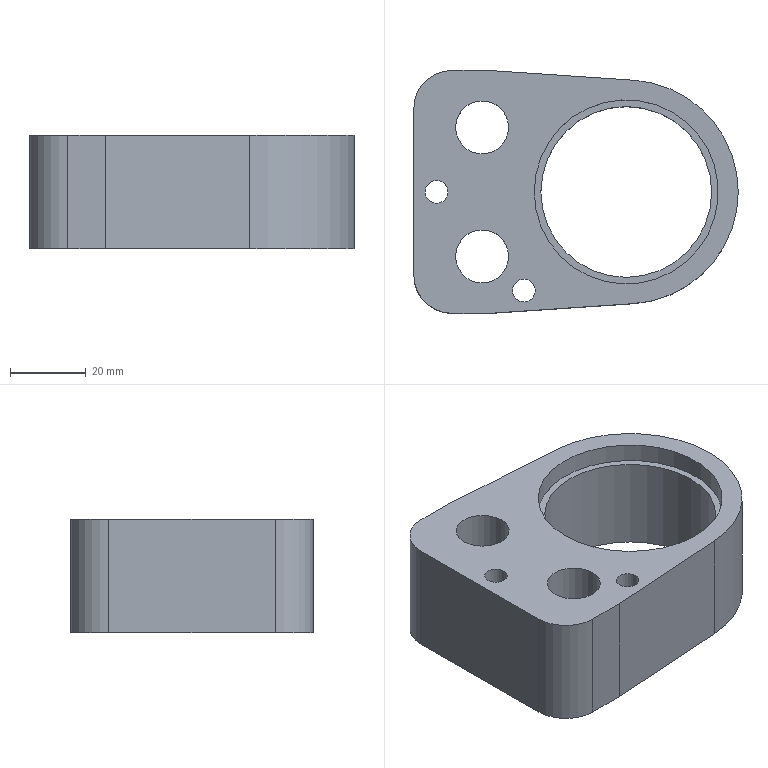Part | NX | features solid 2 | 1 solid | 25 faces | box 85.5 x 64 x 30 mm | volume 80178 mm3 | cylinder 13 | plane 12 | commonest cylinder face diameters 6 x2 8 x2 14 x2 19 x2 20 x2 45 x1
STEP:
#1=CARTESIAN_POINT('',(49.,45.006,17.));
#2=VERTEX_POINT('',#1);
#3=CARTESIAN_POINT('',(45.,45.006,17.));
#4=DIRECTION('',(0.,0.,1.));
#5=DIRECTION('',(1.,0.,0.));
#6=AXIS2_PLACEMENT_3D('',#3,#4,#5);
#7=CIRCLE('',#6,4.);
#8=EDGE_CURVE('',#2,#2,#7,.F.);
#9=ORIENTED_EDGE('',*,*,#8,.F.);
#10=EDGE_LOOP('',(#9));
#11=FACE_BOUND('',#10,.T.);
#12=CARTESIAN_POINT('',(47.5,28.006,17.));
#13=VERTEX_POINT('',#12);
#14=CARTESIAN_POINT('',(57.,28.006,17.));
#15=DIRECTION('',(0.,0.,-1.));
#16=DIRECTION('',(-1.,0.,0.));
#17=AXIS2_PLACEMENT_3D('',#14,#15,#16);
#18=CIRCLE('',#17,9.5);
#19=EDGE_CURVE('',#13,#13,#18,.T.);
#20=ORIENTED_EDGE('',*,*,#19,.F.);
#21=EDGE_LOOP('',(#20));
#22=FACE_BOUND('',#21,.T.);
#23=CARTESIAN_POINT('',(47.5,62.006,17.));
#24=VERTEX_POINT('',#23);
#25=CARTESIAN_POINT('',(57.,62.006,17.));
#26=DIRECTION('',(0.,0.,-1.));
#27=DIRECTION('',(-1.,0.,0.));
#28=AXIS2_PLACEMENT_3D('',#25,#26,#27);
#29=CIRCLE('',#28,9.5);
#30=EDGE_CURVE('',#24,#24,#29,.T.);
#31=ORIENTED_EDGE('',*,*,#30,.F.);
#32=EDGE_LOOP('',(#31));
#33=FACE_BOUND('',#32,.T.);
#34=CARTESIAN_POINT('',(117.5,45.006,17.));
#35=VERTEX_POINT('',#34);
#36=CARTESIAN_POINT('',(95.,45.006,17.));
#37=DIRECTION('',(0.,0.,1.));
#38=DIRECTION('',(1.,0.,0.));
#39=AXIS2_PLACEMENT_3D('',#36,#37,#38);
#40=CIRCLE('',#39,22.5);
#41=EDGE_CURVE('',#35,#35,#40,.T.);
#42=ORIENTED_EDGE('',*,*,#41,.T.);
#43=EDGE_LOOP('',(#42));
#44=FACE_BOUND('',#43,.T.);
#45=CARTESIAN_POINT('',(96.989,74.439,17.));
#46=VERTEX_POINT('',#45);
#47=CARTESIAN_POINT('',(59.,77.006,17.));
#48=VERTEX_POINT('',#47);
#49=CARTESIAN_POINT('',(96.989,74.439,17.));
#50=DIRECTION('',(-0.9977,0.06742,0.));
#51=VECTOR('',#50,1000.);
#52=LINE('',#49,#51);
#53=EDGE_CURVE('',#46,#48,#52,.T.);
#54=ORIENTED_EDGE('',*,*,#53,.F.);
#55=CARTESIAN_POINT('',(96.989,15.574,17.));
#56=VERTEX_POINT('',#55);
#57=CARTESIAN_POINT('',(95.,45.006,17.));
#58=DIRECTION('',(0.,0.,-1.));
#59=DIRECTION('',(-1.,0.,0.));
#60=AXIS2_PLACEMENT_3D('',#57,#58,#59);
#61=CIRCLE('',#60,29.5);
#62=EDGE_CURVE('',#46,#56,#61,.T.);
#63=ORIENTED_EDGE('',*,*,#62,.T.);
#64=CARTESIAN_POINT('',(59.,13.006,17.));
#65=VERTEX_POINT('',#64);
#66=CARTESIAN_POINT('',(96.989,15.574,17.));
#67=DIRECTION('',(-0.9977,-0.06742,0.));
#68=VECTOR('',#67,1000.);
#69=LINE('',#66,#68);
#70=EDGE_CURVE('',#56,#65,#69,.T.);
#71=ORIENTED_EDGE('',*,*,#70,.T.);
#72=CARTESIAN_POINT('',(49.,13.006,17.));
#73=VERTEX_POINT('',#72);
#74=CARTESIAN_POINT('',(59.,13.006,17.));
#75=DIRECTION('',(-1.,0.,0.));
#76=VECTOR('',#75,1000.);
#77=LINE('',#74,#76);
#78=EDGE_CURVE('',#65,#73,#77,.T.);
#79=ORIENTED_EDGE('',*,*,#78,.T.);
#80=CARTESIAN_POINT('',(39.,23.006,17.));
#81=VERTEX_POINT('',#80);
#82=CARTESIAN_POINT('',(49.,23.006,17.));
#83=DIRECTION('',(0.,0.,-1.));
#84=DIRECTION('',(-1.,0.,0.));
#85=AXIS2_PLACEMENT_3D('',#82,#83,#84);
#86=CIRCLE('',#85,10.);
#87=EDGE_CURVE('',#73,#81,#86,.T.);
#88=ORIENTED_EDGE('',*,*,#87,.T.);
#89=CARTESIAN_POINT('',(39.,67.006,17.));
#90=VERTEX_POINT('',#89);
#91=CARTESIAN_POINT('',(39.,67.006,17.));
#92=DIRECTION('',(0.,-1.,0.));
#93=VECTOR('',#92,1000.);
#94=LINE('',#91,#93);
#95=EDGE_CURVE('',#90,#81,#94,.T.);
#96=ORIENTED_EDGE('',*,*,#95,.F.);
#97=CARTESIAN_POINT('',(49.,77.006,17.));
#98=VERTEX_POINT('',#97);
#99=CARTESIAN_POINT('',(49.,67.006,17.));
#100=DIRECTION('',(0.,0.,-1.));
#101=DIRECTION('',(-1.,0.,0.));
#102=AXIS2_PLACEMENT_3D('',#99,#100,#101);
#103=CIRCLE('',#102,10.);
#104=EDGE_CURVE('',#90,#98,#103,.T.);
#105=ORIENTED_EDGE('',*,*,#104,.T.);
#106=CARTESIAN_POINT('',(59.,77.006,17.));
#107=DIRECTION('',(-1.,0.,0.));
#108=VECTOR('',#107,1000.);
#109=LINE('',#106,#108);
#110=EDGE_CURVE('',#48,#98,#109,.T.);
#111=ORIENTED_EDGE('',*,*,#110,.F.);
#112=EDGE_LOOP('',(#54,#63,#71,#79,#88,#96,#105,#111));
#113=FACE_BOUND('',#112,.T.);
#114=CARTESIAN_POINT('',(72.,19.006,17.));
#115=VERTEX_POINT('',#114);
#116=CARTESIAN_POINT('',(68.,19.006,17.));
#117=DIRECTION('',(0.,0.,1.));
#118=DIRECTION('',(1.,0.,0.));
#119=AXIS2_PLACEMENT_3D('',#116,#117,#118);
#120=CIRCLE('',#119,4.);
#121=EDGE_CURVE('',#115,#115,#120,.F.);
#122=ORIENTED_EDGE('',*,*,#121,.F.);
#123=EDGE_LOOP('',(#122));
#124=FACE_BOUND('',#123,.T.);
#125=CARTESIAN_POINT('',(49.,67.006,17.));
#126=DIRECTION('',(0.,0.,-1.));
#127=DIRECTION('',(-1.,0.,0.));
#128=AXIS2_PLACEMENT_3D('',#125,#126,#127);
#129=PLANE('',#128);
#130=ADVANCED_FACE('',(#11,#22,#33,#44,#113,#124),#129,.T.);
#131=CARTESIAN_POINT('',(42.,45.006,47.));
#132=VERTEX_POINT('',#131);
#133=CARTESIAN_POINT('',(45.,45.006,47.));
#134=DIRECTION('',(0.,0.,-1.));
#135=DIRECTION('',(-1.,0.,0.));
#136=AXIS2_PLACEMENT_3D('',#133,#134,#135);
#137=CIRCLE('',#136,3.);
#138=EDGE_CURVE('',#132,#132,#137,.T.);
#139=ORIENTED_EDGE('',*,*,#138,.F.);
#140=EDGE_LOOP('',(#139));
#141=FACE_BOUND('',#140,.T.);
#142=CARTESIAN_POINT('',(42.,45.006,37.));
#143=VERTEX_POINT('',#142);
#144=CARTESIAN_POINT('',(45.,45.006,37.));
#145=DIRECTION('',(0.,0.,-1.));
#146=DIRECTION('',(-1.,0.,0.));
#147=AXIS2_PLACEMENT_3D('',#144,#145,#146);
#148=CIRCLE('',#147,3.);
#149=EDGE_CURVE('',#143,#143,#148,.T.);
#150=ORIENTED_EDGE('',*,*,#149,.T.);
#151=EDGE_LOOP('',(#150));
#152=FACE_BOUND('',#151,.T.);
#153=CARTESIAN_POINT('',(45.,45.006,17.));
#154=DIRECTION('',(0.,0.,1.));
#155=DIRECTION('',(1.,0.,0.));
#156=AXIS2_PLACEMENT_3D('',#153,#154,#155);
#157=CYLINDRICAL_SURFACE('',#156,3.);
#158=ADVANCED_FACE('',(#141,#152),#157,.F.);
#159=CARTESIAN_POINT('',(50.,28.006,47.));
#160=VERTEX_POINT('',#159);
#161=CARTESIAN_POINT('',(57.,28.006,47.));
#162=DIRECTION('',(0.,0.,-1.));
#163=DIRECTION('',(-1.,0.,0.));
#164=AXIS2_PLACEMENT_3D('',#161,#162,#163);
#165=CIRCLE('',#164,7.);
#166=EDGE_CURVE('',#160,#160,#165,.T.);
#167=ORIENTED_EDGE('',*,*,#166,.F.);
#168=EDGE_LOOP('',(#167));
#169=FACE_BOUND('',#168,.T.);
#170=CARTESIAN_POINT('',(50.,28.006,31.));
#171=VERTEX_POINT('',#170);
#172=CARTESIAN_POINT('',(57.,28.006,31.));
#173=DIRECTION('',(0.,0.,-1.));
#174=DIRECTION('',(-1.,0.,0.));
#175=AXIS2_PLACEMENT_3D('',#172,#173,#174);
#176=CIRCLE('',#175,7.);
#177=EDGE_CURVE('',#171,#171,#176,.T.);
#178=ORIENTED_EDGE('',*,*,#177,.T.);
#179=EDGE_LOOP('',(#178));
#180=FACE_BOUND('',#179,.T.);
#181=CARTESIAN_POINT('',(57.,28.006,17.));
#182=DIRECTION('',(0.,0.,1.));
#183=DIRECTION('',(1.,0.,0.));
#184=AXIS2_PLACEMENT_3D('',#181,#182,#183);
#185=CYLINDRICAL_SURFACE('',#184,7.);
#186=ADVANCED_FACE('',(#169,#180),#185,.F.);
#187=CARTESIAN_POINT('',(50.,62.006,47.));
#188=VERTEX_POINT('',#187);
#189=CARTESIAN_POINT('',(57.,62.006,47.));
#190=DIRECTION('',(0.,0.,-1.));
#191=DIRECTION('',(-1.,0.,0.));
#192=AXIS2_PLACEMENT_3D('',#189,#190,#191);
#193=CIRCLE('',#192,7.);
#194=EDGE_CURVE('',#188,#188,#193,.T.);
#195=ORIENTED_EDGE('',*,*,#194,.F.);
#196=EDGE_LOOP('',(#195));
#197=FACE_BOUND('',#196,.T.);
#198=CARTESIAN_POINT('',(50.,62.006,31.));
#199=VERTEX_POINT('',#198);
#200=CARTESIAN_POINT('',(57.,62.006,31.));
#201=DIRECTION('',(0.,0.,-1.));
#202=DIRECTION('',(-1.,0.,0.));
#203=AXIS2_PLACEMENT_3D('',#200,#201,#202);
#204=CIRCLE('',#203,7.);
#205=EDGE_CURVE('',#199,#199,#204,.T.);
#206=ORIENTED_EDGE('',*,*,#205,.T.);
#207=EDGE_LOOP('',(#206));
#208=FACE_BOUND('',#207,.T.);
#209=CARTESIAN_POINT('',(57.,62.006,17.));
#210=DIRECTION('',(0.,0.,1.));
#211=DIRECTION('',(1.,0.,0.));
#212=AXIS2_PLACEMENT_3D('',#209,#210,#211);
#213=CYLINDRICAL_SURFACE('',#212,7.);
#214=ADVANCED_FACE('',(#197,#208),#213,.F.);
#215=CARTESIAN_POINT('',(65.,19.006,47.));
#216=VERTEX_POINT('',#215);
#217=CARTESIAN_POINT('',(68.,19.006,47.));
#218=DIRECTION('',(0.,0.,-1.));
#219=DIRECTION('',(-1.,0.,0.));
#220=AXIS2_PLACEMENT_3D('',#217,#218,#219);
#221=CIRCLE('',#220,3.);
#222=EDGE_CURVE('',#216,#216,#221,.T.);
#223=ORIENTED_EDGE('',*,*,#222,.T.);
#224=EDGE_LOOP('',(#223));
#225=FACE_BOUND('',#224,.T.);
#226=ORIENTED_EDGE('',*,*,#166,.T.);
#227=EDGE_LOOP('',(#226));
#228=FACE_BOUND('',#227,.T.);
#229=CARTESIAN_POINT('',(96.989,74.439,47.));
#230=VERTEX_POINT('',#229);
#231=CARTESIAN_POINT('',(59.,77.006,47.));
#232=VERTEX_POINT('',#231);
#233=CARTESIAN_POINT('',(96.989,74.439,47.));
#234=DIRECTION('',(-0.9977,0.06742,0.));
#235=VECTOR('',#234,1000.);
#236=LINE('',#233,#235);
#237=EDGE_CURVE('',#230,#232,#236,.T.);
#238=ORIENTED_EDGE('',*,*,#237,.T.);
#239=CARTESIAN_POINT('',(49.,77.006,47.));
#240=VERTEX_POINT('',#239);
#241=CARTESIAN_POINT('',(59.,77.006,47.));
#242=DIRECTION('',(-1.,0.,0.));
#243=VECTOR('',#242,1000.);
#244=LINE('',#241,#243);
#245=EDGE_CURVE('',#232,#240,#244,.T.);
#246=ORIENTED_EDGE('',*,*,#245,.T.);
#247=CARTESIAN_POINT('',(39.,67.006,47.));
#248=VERTEX_POINT('',#247);
#249=CARTESIAN_POINT('',(49.,67.006,47.));
#250=DIRECTION('',(0.,0.,-1.));
#251=DIRECTION('',(-1.,0.,0.));
#252=AXIS2_PLACEMENT_3D('',#249,#250,#251);
#253=CIRCLE('',#252,10.);
#254=EDGE_CURVE('',#248,#240,#253,.T.);
#255=ORIENTED_EDGE('',*,*,#254,.F.);
#256=CARTESIAN_POINT('',(39.,23.006,47.));
#257=VERTEX_POINT('',#256);
#258=CARTESIAN_POINT('',(39.,67.006,47.));
#259=DIRECTION('',(0.,-1.,0.));
#260=VECTOR('',#259,1000.);
#261=LINE('',#258,#260);
#262=EDGE_CURVE('',#248,#257,#261,.T.);
#263=ORIENTED_EDGE('',*,*,#262,.T.);
#264=CARTESIAN_POINT('',(49.,13.006,47.));
#265=VERTEX_POINT('',#264);
#266=CARTESIAN_POINT('',(49.,23.006,47.));
#267=DIRECTION('',(0.,0.,-1.));
#268=DIRECTION('',(-1.,0.,0.));
#269=AXIS2_PLACEMENT_3D('',#266,#267,#268);
#270=CIRCLE('',#269,10.);
#271=EDGE_CURVE('',#265,#257,#270,.T.);
#272=ORIENTED_EDGE('',*,*,#271,.F.);
#273=CARTESIAN_POINT('',(59.,13.006,47.));
#274=VERTEX_POINT('',#273);
#275=CARTESIAN_POINT('',(59.,13.006,47.));
#276=DIRECTION('',(-1.,0.,0.));
#277=VECTOR('',#276,1000.);
#278=LINE('',#275,#277);
#279=EDGE_CURVE('',#274,#265,#278,.T.);
#280=ORIENTED_EDGE('',*,*,#279,.F.);
#281=CARTESIAN_POINT('',(96.989,15.574,47.));
#282=VERTEX_POINT('',#281);
#283=CARTESIAN_POINT('',(96.989,15.574,47.));
#284=DIRECTION('',(-0.9977,-0.06742,0.));
#285=VECTOR('',#284,1000.);
#286=LINE('',#283,#285);
#287=EDGE_CURVE('',#282,#274,#286,.T.);
#288=ORIENTED_EDGE('',*,*,#287,.F.);
#289=CARTESIAN_POINT('',(95.,45.006,47.));
#290=DIRECTION('',(0.,0.,-1.));
#291=DIRECTION('',(-1.,0.,0.));
#292=AXIS2_PLACEMENT_3D('',#289,#290,#291);
#293=CIRCLE('',#292,29.5);
#294=EDGE_CURVE('',#230,#282,#293,.T.);
#295=ORIENTED_EDGE('',*,*,#294,.F.);
#296=EDGE_LOOP('',(#238,#246,#255,#263,#272,#280,#288,#295));
#297=FACE_BOUND('',#296,.T.);
#298=CARTESIAN_POINT('',(70.75,45.006,47.));
#299=VERTEX_POINT('',#298);
#300=CARTESIAN_POINT('',(95.,45.006,47.));
#301=DIRECTION('',(0.,0.,-1.));
#302=DIRECTION('',(-1.,0.,0.));
#303=AXIS2_PLACEMENT_3D('',#300,#301,#302);
#304=CIRCLE('',#303,24.25);
#305=EDGE_CURVE('',#299,#299,#304,.T.);
#306=ORIENTED_EDGE('',*,*,#305,.T.);
#307=EDGE_LOOP('',(#306));
#308=FACE_BOUND('',#307,.T.);
#309=ORIENTED_EDGE('',*,*,#194,.T.);
#310=EDGE_LOOP('',(#309));
#311=FACE_BOUND('',#310,.T.);
#312=ORIENTED_EDGE('',*,*,#138,.T.);
#313=EDGE_LOOP('',(#312));
#314=FACE_BOUND('',#313,.T.);
#315=CARTESIAN_POINT('',(49.,67.006,47.));
#316=DIRECTION('',(0.,0.,-1.));
#317=DIRECTION('',(-1.,0.,0.));
#318=AXIS2_PLACEMENT_3D('',#315,#316,#317);
#319=PLANE('',#318);
#320=ADVANCED_FACE('',(#225,#228,#297,#308,#311,#314),#319,.F.);
#321=ORIENTED_EDGE('',*,*,#237,.F.);
#322=CARTESIAN_POINT('',(96.989,74.439,17.));
#323=DIRECTION('',(0.,0.,1.));
#324=VECTOR('',#323,1000.);
#325=LINE('',#322,#324);
#326=EDGE_CURVE('',#46,#230,#325,.T.);
#327=ORIENTED_EDGE('',*,*,#326,.F.);
#328=ORIENTED_EDGE('',*,*,#53,.T.);
#329=CARTESIAN_POINT('',(59.,77.006,17.));
#330=DIRECTION('',(0.,0.,1.));
#331=VECTOR('',#330,1000.);
#332=LINE('',#329,#331);
#333=EDGE_CURVE('',#48,#232,#332,.T.);
#334=ORIENTED_EDGE('',*,*,#333,.T.);
#335=EDGE_LOOP('',(#321,#327,#328,#334));
#336=FACE_BOUND('',#335,.T.);
#337=CARTESIAN_POINT('',(96.989,74.439,17.));
#338=DIRECTION('',(0.06742,0.9977,0.));
#339=DIRECTION('',(-0.9977,0.06742,0.));
#340=AXIS2_PLACEMENT_3D('',#337,#338,#339);
#341=PLANE('',#340);
#342=ADVANCED_FACE('',(#336),#341,.T.);
#343=ORIENTED_EDGE('',*,*,#245,.F.);
#344=ORIENTED_EDGE('',*,*,#333,.F.);
#345=ORIENTED_EDGE('',*,*,#110,.T.);
#346=CARTESIAN_POINT('',(49.,77.006,17.));
#347=DIRECTION('',(0.,0.,1.));
#348=VECTOR('',#347,1000.);
#349=LINE('',#346,#348);
#350=EDGE_CURVE('',#98,#240,#349,.T.);
#351=ORIENTED_EDGE('',*,*,#350,.T.);
#352=EDGE_LOOP('',(#343,#344,#345,#351));
#353=FACE_BOUND('',#352,.T.);
#354=CARTESIAN_POINT('',(59.,77.006,17.));
#355=DIRECTION('',(0.,1.,0.));
#356=DIRECTION('',(0.,0.,1.));
#357=AXIS2_PLACEMENT_3D('',#354,#355,#356);
#358=PLANE('',#357);
#359=ADVANCED_FACE('',(#353),#358,.T.);
#360=ORIENTED_EDGE('',*,*,#254,.T.);
#361=ORIENTED_EDGE('',*,*,#350,.F.);
#362=ORIENTED_EDGE('',*,*,#104,.F.);
#363=CARTESIAN_POINT('',(39.,67.006,17.));
#364=DIRECTION('',(0.,0.,1.));
#365=VECTOR('',#364,1000.);
#366=LINE('',#363,#365);
#367=EDGE_CURVE('',#90,#248,#366,.T.);
#368=ORIENTED_EDGE('',*,*,#367,.T.);
#369=EDGE_LOOP('',(#360,#361,#362,#368));
#370=FACE_BOUND('',#369,.T.);
#371=CARTESIAN_POINT('',(49.,67.006,17.));
#372=DIRECTION('',(0.,0.,1.));
#373=DIRECTION('',(1.,0.,0.));
#374=AXIS2_PLACEMENT_3D('',#371,#372,#373);
#375=CYLINDRICAL_SURFACE('',#374,10.);
#376=ADVANCED_FACE('',(#370),#375,.T.);
#377=ORIENTED_EDGE('',*,*,#262,.F.);
#378=ORIENTED_EDGE('',*,*,#367,.F.);
#379=ORIENTED_EDGE('',*,*,#95,.T.);
#380=CARTESIAN_POINT('',(39.,23.006,17.));
#381=DIRECTION('',(0.,0.,1.));
#382=VECTOR('',#381,1000.);
#383=LINE('',#380,#382);
#384=EDGE_CURVE('',#81,#257,#383,.T.);
#385=ORIENTED_EDGE('',*,*,#384,.T.);
#386=EDGE_LOOP('',(#377,#378,#379,#385));
#387=FACE_BOUND('',#386,.T.);
#388=CARTESIAN_POINT('',(39.,67.006,17.));
#389=DIRECTION('',(-1.,0.,0.));
#390=DIRECTION('',(0.,-1.,0.));
#391=AXIS2_PLACEMENT_3D('',#388,#389,#390);
#392=PLANE('',#391);
#393=ADVANCED_FACE('',(#387),#392,.T.);
#394=ORIENTED_EDGE('',*,*,#271,.T.);
#395=ORIENTED_EDGE('',*,*,#384,.F.);
#396=ORIENTED_EDGE('',*,*,#87,.F.);
#397=CARTESIAN_POINT('',(49.,13.006,17.));
#398=DIRECTION('',(0.,0.,1.));
#399=VECTOR('',#398,1000.);
#400=LINE('',#397,#399);
#401=EDGE_CURVE('',#73,#265,#400,.T.);
#402=ORIENTED_EDGE('',*,*,#401,.T.);
#403=EDGE_LOOP('',(#394,#395,#396,#402));
#404=FACE_BOUND('',#403,.T.);
#405=CARTESIAN_POINT('',(49.,23.006,17.));
#406=DIRECTION('',(0.,0.,1.));
#407=DIRECTION('',(1.,0.,0.));
#408=AXIS2_PLACEMENT_3D('',#405,#406,#407);
#409=CYLINDRICAL_SURFACE('',#408,10.);
#410=ADVANCED_FACE('',(#404),#409,.T.);
#411=ORIENTED_EDGE('',*,*,#279,.T.);
#412=ORIENTED_EDGE('',*,*,#401,.F.);
#413=ORIENTED_EDGE('',*,*,#78,.F.);
#414=CARTESIAN_POINT('',(59.,13.006,17.));
#415=DIRECTION('',(0.,0.,1.));
#416=VECTOR('',#415,1000.);
#417=LINE('',#414,#416);
#418=EDGE_CURVE('',#65,#274,#417,.T.);
#419=ORIENTED_EDGE('',*,*,#418,.T.);
#420=EDGE_LOOP('',(#411,#412,#413,#419));
#421=FACE_BOUND('',#420,.T.);
#422=CARTESIAN_POINT('',(59.,13.006,17.));
#423=DIRECTION('',(0.,1.,0.));
#424=DIRECTION('',(-1.,0.,0.));
#425=AXIS2_PLACEMENT_3D('',#422,#423,#424);
#426=PLANE('',#425);
#427=ADVANCED_FACE('',(#421),#426,.F.);
#428=ORIENTED_EDGE('',*,*,#287,.T.);
#429=ORIENTED_EDGE('',*,*,#418,.F.);
#430=ORIENTED_EDGE('',*,*,#70,.F.);
#431=CARTESIAN_POINT('',(96.989,15.574,17.));
#432=DIRECTION('',(0.,0.,1.));
#433=VECTOR('',#432,1000.);
#434=LINE('',#431,#433);
#435=EDGE_CURVE('',#56,#282,#434,.T.);
#436=ORIENTED_EDGE('',*,*,#435,.T.);
#437=EDGE_LOOP('',(#428,#429,#430,#436));
#438=FACE_BOUND('',#437,.T.);
#439=CARTESIAN_POINT('',(96.989,15.574,17.));
#440=DIRECTION('',(-0.06742,0.9977,0.));
#441=DIRECTION('',(-0.9977,-0.06742,0.));
#442=AXIS2_PLACEMENT_3D('',#439,#440,#441);
#443=PLANE('',#442);
#444=ADVANCED_FACE('',(#438),#443,.F.);
#445=ORIENTED_EDGE('',*,*,#294,.T.);
#446=ORIENTED_EDGE('',*,*,#435,.F.);
#447=ORIENTED_EDGE('',*,*,#62,.F.);
#448=ORIENTED_EDGE('',*,*,#326,.T.);
#449=EDGE_LOOP('',(#445,#446,#447,#448));
#450=FACE_BOUND('',#449,.T.);
#451=CARTESIAN_POINT('',(95.,45.006,17.));
#452=DIRECTION('',(0.,0.,1.));
#453=DIRECTION('',(1.,0.,0.));
#454=AXIS2_PLACEMENT_3D('',#451,#452,#453);
#455=CYLINDRICAL_SURFACE('',#454,29.5);
#456=ADVANCED_FACE('',(#450),#455,.T.);
#457=CARTESIAN_POINT('',(72.5,45.006,42.));
#458=VERTEX_POINT('',#457);
#459=CARTESIAN_POINT('',(95.,45.006,42.));
#460=DIRECTION('',(0.,0.,-1.));
#461=DIRECTION('',(-1.,0.,0.));
#462=AXIS2_PLACEMENT_3D('',#459,#460,#461);
#463=CIRCLE('',#462,22.5);
#464=EDGE_CURVE('',#458,#458,#463,.F.);
#465=ORIENTED_EDGE('',*,*,#464,.T.);
#466=EDGE_LOOP('',(#465));
#467=FACE_BOUND('',#466,.T.);
#468=ORIENTED_EDGE('',*,*,#41,.F.);
#469=EDGE_LOOP('',(#468));
#470=FACE_BOUND('',#469,.T.);
#471=CARTESIAN_POINT('',(95.,45.006,17.));
#472=DIRECTION('',(0.,0.,1.));
#473=DIRECTION('',(1.,0.,0.));
#474=AXIS2_PLACEMENT_3D('',#471,#472,#473);
#475=CYLINDRICAL_SURFACE('',#474,22.5);
#476=ADVANCED_FACE('',(#467,#470),#475,.F.);
#477=CARTESIAN_POINT('',(70.75,45.006,42.));
#478=VERTEX_POINT('',#477);
#479=CARTESIAN_POINT('',(95.,45.006,42.));
#480=DIRECTION('',(0.,0.,-1.));
#481=DIRECTION('',(-1.,0.,0.));
#482=AXIS2_PLACEMENT_3D('',#479,#480,#481);
#483=CIRCLE('',#482,24.25);
#484=EDGE_CURVE('',#478,#478,#483,.T.);
#485=ORIENTED_EDGE('',*,*,#484,.F.);
#486=EDGE_LOOP('',(#485));
#487=FACE_BOUND('',#486,.T.);
#488=ORIENTED_EDGE('',*,*,#464,.F.);
#489=EDGE_LOOP('',(#488));
#490=FACE_BOUND('',#489,.T.);
#491=CARTESIAN_POINT('',(95.,45.006,42.));
#492=DIRECTION('',(0.,0.,-1.));
#493=DIRECTION('',(-1.,0.,0.));
#494=AXIS2_PLACEMENT_3D('',#491,#492,#493);
#495=PLANE('',#494);
#496=ADVANCED_FACE('',(#487,#490),#495,.F.);
#497=ORIENTED_EDGE('',*,*,#484,.T.);
#498=EDGE_LOOP('',(#497));
#499=FACE_BOUND('',#498,.T.);
#500=ORIENTED_EDGE('',*,*,#305,.F.);
#501=EDGE_LOOP('',(#500));
#502=FACE_BOUND('',#501,.T.);
#503=CARTESIAN_POINT('',(95.,45.006,42.));
#504=DIRECTION('',(0.,0.,1.));
#505=DIRECTION('',(1.,0.,0.));
#506=AXIS2_PLACEMENT_3D('',#503,#504,#505);
#507=CYLINDRICAL_SURFACE('',#506,24.25);
#508=ADVANCED_FACE('',(#499,#502),#507,.F.);
#509=CARTESIAN_POINT('',(65.,19.006,37.));
#510=VERTEX_POINT('',#509);
#511=CARTESIAN_POINT('',(68.,19.006,37.));
#512=DIRECTION('',(0.,0.,-1.));
#513=DIRECTION('',(-1.,0.,0.));
#514=AXIS2_PLACEMENT_3D('',#511,#512,#513);
#515=CIRCLE('',#514,3.);
#516=EDGE_CURVE('',#510,#510,#515,.T.);
#517=ORIENTED_EDGE('',*,*,#516,.T.);
#518=EDGE_LOOP('',(#517));
#519=FACE_BOUND('',#518,.T.);
#520=ORIENTED_EDGE('',*,*,#222,.F.);
#521=EDGE_LOOP('',(#520));
#522=FACE_BOUND('',#521,.T.);
#523=CARTESIAN_POINT('',(68.,19.006,17.));
#524=DIRECTION('',(0.,0.,1.));
#525=DIRECTION('',(1.,0.,0.));
#526=AXIS2_PLACEMENT_3D('',#523,#524,#525);
#527=CYLINDRICAL_SURFACE('',#526,3.);
#528=ADVANCED_FACE('',(#519,#522),#527,.F.);
#529=CARTESIAN_POINT('',(47.5,62.006,31.));
#530=VERTEX_POINT('',#529);
#531=CARTESIAN_POINT('',(57.,62.006,31.));
#532=DIRECTION('',(0.,0.,-1.));
#533=DIRECTION('',(-1.,0.,0.));
#534=AXIS2_PLACEMENT_3D('',#531,#532,#533);
#535=CIRCLE('',#534,9.5);
#536=EDGE_CURVE('',#530,#530,#535,.T.);
#537=ORIENTED_EDGE('',*,*,#536,.F.);
#538=EDGE_LOOP('',(#537));
#539=FACE_BOUND('',#538,.T.);
#540=ORIENTED_EDGE('',*,*,#30,.T.);
#541=EDGE_LOOP('',(#540));
#542=FACE_BOUND('',#541,.T.);
#543=CARTESIAN_POINT('',(57.,62.006,31.));
#544=DIRECTION('',(0.,0.,-1.));
#545=DIRECTION('',(-1.,0.,0.));
#546=AXIS2_PLACEMENT_3D('',#543,#544,#545);
#547=CYLINDRICAL_SURFACE('',#546,9.5);
#548=ADVANCED_FACE('',(#539,#542),#547,.F.);
#549=ORIENTED_EDGE('',*,*,#205,.F.);
#550=EDGE_LOOP('',(#549));
#551=FACE_BOUND('',#550,.T.);
#552=ORIENTED_EDGE('',*,*,#536,.T.);
#553=EDGE_LOOP('',(#552));
#554=FACE_BOUND('',#553,.T.);
#555=CARTESIAN_POINT('',(57.,62.006,31.));
#556=DIRECTION('',(0.,0.,-1.));
#557=DIRECTION('',(-1.,0.,0.));
#558=AXIS2_PLACEMENT_3D('',#555,#556,#557);
#559=PLANE('',#558);
#560=ADVANCED_FACE('',(#551,#554),#559,.T.);
#561=CARTESIAN_POINT('',(47.5,28.006,31.));
#562=VERTEX_POINT('',#561);
#563=CARTESIAN_POINT('',(57.,28.006,31.));
#564=DIRECTION('',(0.,0.,-1.));
#565=DIRECTION('',(-1.,0.,0.));
#566=AXIS2_PLACEMENT_3D('',#563,#564,#565);
#567=CIRCLE('',#566,9.5);
#568=EDGE_CURVE('',#562,#562,#567,.T.);
#569=ORIENTED_EDGE('',*,*,#568,.F.);
#570=EDGE_LOOP('',(#569));
#571=FACE_BOUND('',#570,.T.);
#572=ORIENTED_EDGE('',*,*,#19,.T.);
#573=EDGE_LOOP('',(#572));
#574=FACE_BOUND('',#573,.T.);
#575=CARTESIAN_POINT('',(57.,28.006,31.));
#576=DIRECTION('',(0.,0.,-1.));
#577=DIRECTION('',(-1.,0.,0.));
#578=AXIS2_PLACEMENT_3D('',#575,#576,#577);
#579=CYLINDRICAL_SURFACE('',#578,9.5);
#580=ADVANCED_FACE('',(#571,#574),#579,.F.);
#581=ORIENTED_EDGE('',*,*,#177,.F.);
#582=EDGE_LOOP('',(#581));
#583=FACE_BOUND('',#582,.T.);
#584=ORIENTED_EDGE('',*,*,#568,.T.);
#585=EDGE_LOOP('',(#584));
#586=FACE_BOUND('',#585,.T.);
#587=CARTESIAN_POINT('',(57.,28.006,31.));
#588=DIRECTION('',(0.,0.,-1.));
#589=DIRECTION('',(-1.,0.,0.));
#590=AXIS2_PLACEMENT_3D('',#587,#588,#589);
#591=PLANE('',#590);
#592=ADVANCED_FACE('',(#583,#586),#591,.T.);
#593=ORIENTED_EDGE('',*,*,#149,.F.);
#594=EDGE_LOOP('',(#593));
#595=FACE_BOUND('',#594,.T.);
#596=CARTESIAN_POINT('',(49.,45.006,37.));
#597=VERTEX_POINT('',#596);
#598=CARTESIAN_POINT('',(45.,45.006,37.));
#599=DIRECTION('',(0.,0.,1.));
#600=DIRECTION('',(1.,0.,0.));
#601=AXIS2_PLACEMENT_3D('',#598,#599,#600);
#602=CIRCLE('',#601,4.);
#603=EDGE_CURVE('',#597,#597,#602,.F.);
#604=ORIENTED_EDGE('',*,*,#603,.T.);
#605=EDGE_LOOP('',(#604));
#606=FACE_BOUND('',#605,.T.);
#607=CARTESIAN_POINT('',(45.,45.006,37.));
#608=DIRECTION('',(0.,0.,1.));
#609=DIRECTION('',(1.,0.,0.));
#610=AXIS2_PLACEMENT_3D('',#607,#608,#609);
#611=PLANE('',#610);
#612=ADVANCED_FACE('',(#595,#606),#611,.F.);
#613=ORIENTED_EDGE('',*,*,#603,.F.);
#614=EDGE_LOOP('',(#613));
#615=FACE_BOUND('',#614,.T.);
#616=ORIENTED_EDGE('',*,*,#8,.T.);
#617=EDGE_LOOP('',(#616));
#618=FACE_BOUND('',#617,.T.);
#619=CARTESIAN_POINT('',(45.,45.006,17.));
#620=DIRECTION('',(0.,0.,1.));
#621=DIRECTION('',(1.,0.,0.));
#622=AXIS2_PLACEMENT_3D('',#619,#620,#621);
#623=CYLINDRICAL_SURFACE('',#622,4.);
#624=ADVANCED_FACE('',(#615,#618),#623,.F.);
#625=ORIENTED_EDGE('',*,*,#516,.F.);
#626=EDGE_LOOP('',(#625));
#627=FACE_BOUND('',#626,.T.);
#628=CARTESIAN_POINT('',(72.,19.006,37.));
#629=VERTEX_POINT('',#628);
#630=CARTESIAN_POINT('',(68.,19.006,37.));
#631=DIRECTION('',(0.,0.,1.));
#632=DIRECTION('',(1.,0.,0.));
#633=AXIS2_PLACEMENT_3D('',#630,#631,#632);
#634=CIRCLE('',#633,4.);
#635=EDGE_CURVE('',#629,#629,#634,.F.);
#636=ORIENTED_EDGE('',*,*,#635,.T.);
#637=EDGE_LOOP('',(#636));
#638=FACE_BOUND('',#637,.T.);
#639=CARTESIAN_POINT('',(68.,19.006,37.));
#640=DIRECTION('',(0.,0.,1.));
#641=DIRECTION('',(1.,0.,0.));
#642=AXIS2_PLACEMENT_3D('',#639,#640,#641);
#643=PLANE('',#642);
#644=ADVANCED_FACE('',(#627,#638),#643,.F.);
#645=ORIENTED_EDGE('',*,*,#635,.F.);
#646=EDGE_LOOP('',(#645));
#647=FACE_BOUND('',#646,.T.);
#648=ORIENTED_EDGE('',*,*,#121,.T.);
#649=EDGE_LOOP('',(#648));
#650=FACE_BOUND('',#649,.T.);
#651=CARTESIAN_POINT('',(68.,19.006,17.));
#652=DIRECTION('',(0.,0.,1.));
#653=DIRECTION('',(1.,0.,0.));
#654=AXIS2_PLACEMENT_3D('',#651,#652,#653);
#655=CYLINDRICAL_SURFACE('',#654,4.);
#656=ADVANCED_FACE('',(#647,#650),#655,.F.);
#657=CLOSED_SHELL('',(#130,#158,#186,#214,#320,#342,#359,#376,#393,#410,#427,#444,#456,#476,#496,#508,#528,#548,#560,#580,#592,#612,#624,#644,#656));
#658=MANIFOLD_SOLID_BREP('',#657);
#659=(LENGTH_UNIT()NAMED_UNIT(*)SI_UNIT(.MILLI.,.METRE.));
#660=UNCERTAINTY_MEASURE_WITH_UNIT(LENGTH_MEASURE(0.00001),#659,'','');
#661=(NAMED_UNIT(*)PLANE_ANGLE_UNIT()SI_UNIT($,.RADIAN.));
#662=(NAMED_UNIT(*)SI_UNIT($,.STERADIAN.)SOLID_ANGLE_UNIT());
#663=(GEOMETRIC_REPRESENTATION_CONTEXT(3)GLOBAL_UNCERTAINTY_ASSIGNED_CONTEXT((#660))GLOBAL_UNIT_ASSIGNED_CONTEXT((#659,#661,#662))REPRESENTATION_CONTEXT('',''));
#664=ADVANCED_BREP_SHAPE_REPRESENTATION('',(#658),#663);